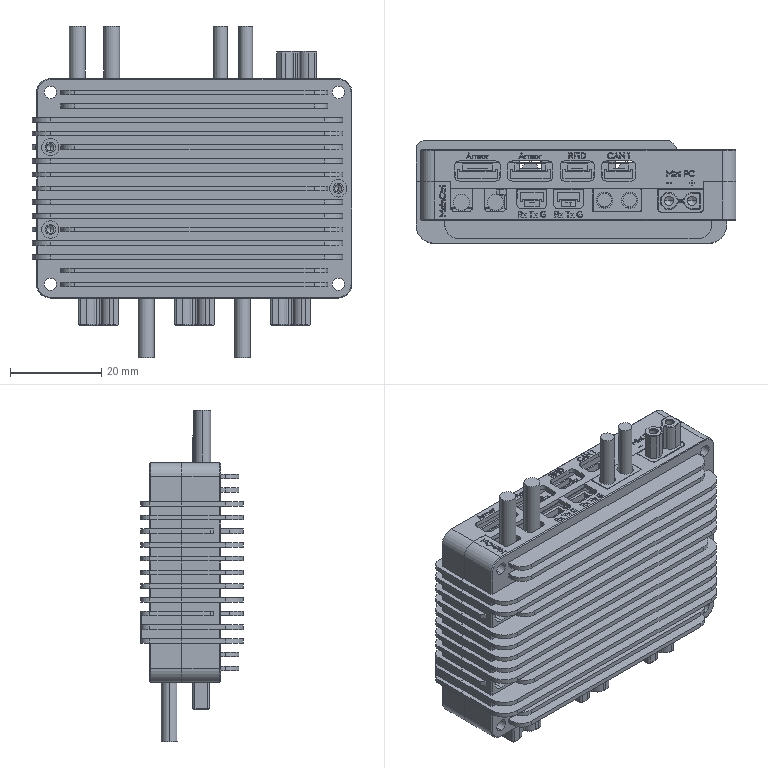Part | SolidWorks | features BaseBody 37 | 37 solids | 7106 faces | volume 27803 mm3 | plane 4212 | spline 1684 | cylinder 1072 | cone 122 | torus 16 | commonest cylinder face diameters 1 x131 2.5 x123 2 x100 3.5 x94 1.4 x64 0.9 x48